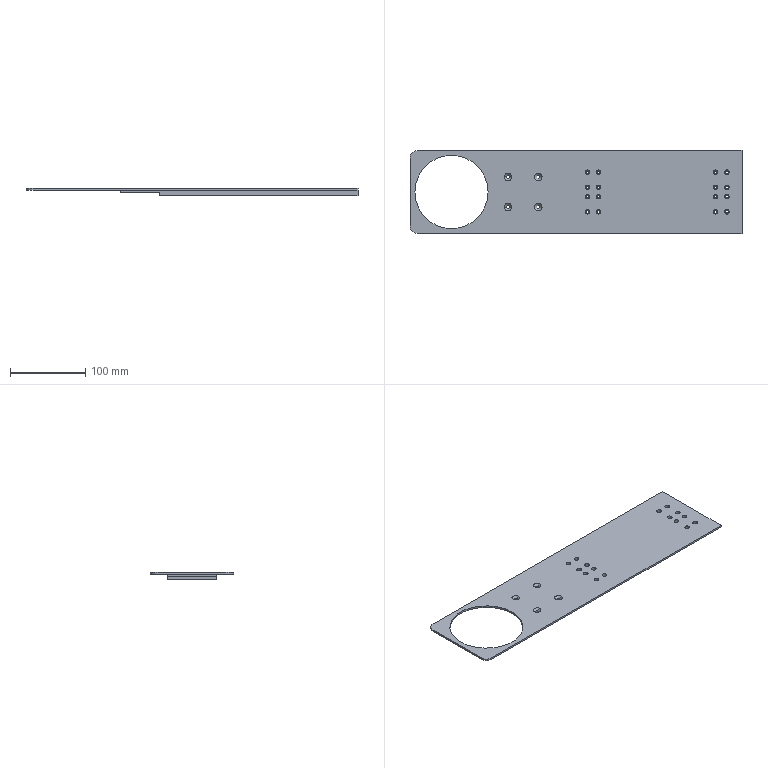Part | STEP file | PN_0009 Push plate | 1 solid | 112 faces | box 440 x 110 x 10 mm | volume 235414 mm3 | cylinder 76 | plane 28 | cone 8 | commonest cylinder face diameters 3.4 x32 6 x32 4.5 x8 20 x2 97 x2